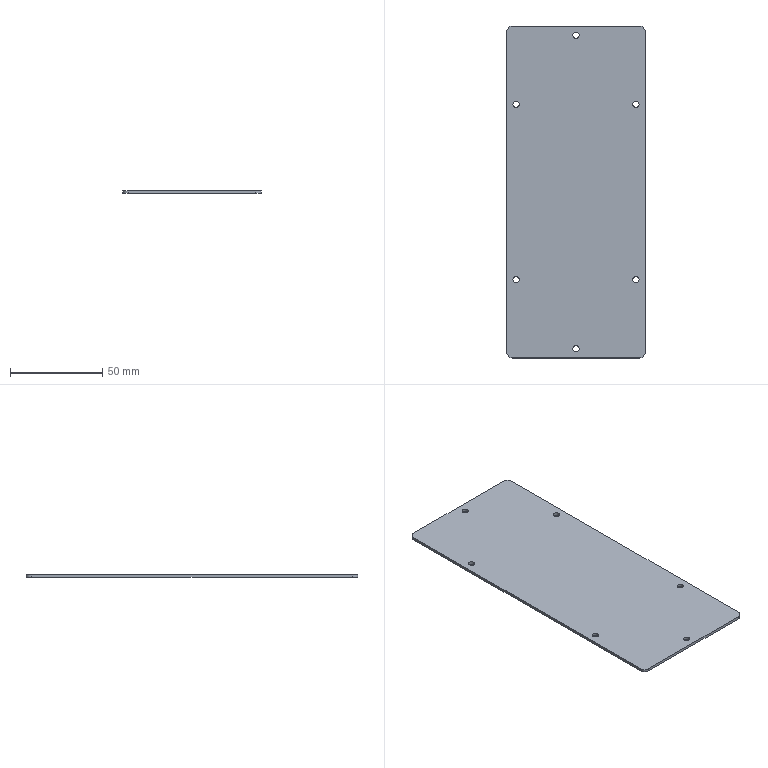Part | NX | 1 solid | 16 faces | box 75 x 180 x 1.5 mm | volume 20157 mm3 | cylinder 10 | plane 6 | commonest cylinder face diameters 3.4 x6 6 x4
STEP:
#1=CARTESIAN_POINT('',(-34.2,47.5,0.));
#2=VERTEX_POINT('',#1);
#3=CARTESIAN_POINT('',(-32.5,47.5,0.));
#4=DIRECTION('',(0.,0.,-1.));
#5=DIRECTION('',(-1.,0.,0.));
#6=AXIS2_PLACEMENT_3D('',#3,#4,#5);
#7=CIRCLE('',#6,1.7);
#8=EDGE_CURVE('',#2,#2,#7,.T.);
#9=ORIENTED_EDGE('',*,*,#8,.F.);
#10=EDGE_LOOP('',(#9));
#11=FACE_BOUND('',#10,.T.);
#12=CARTESIAN_POINT('',(-1.7,-85.,0.));
#13=VERTEX_POINT('',#12);
#14=CARTESIAN_POINT('',(0.,-85.,0.));
#15=DIRECTION('',(0.,0.,-1.));
#16=DIRECTION('',(-1.,0.,0.));
#17=AXIS2_PLACEMENT_3D('',#14,#15,#16);
#18=CIRCLE('',#17,1.7);
#19=EDGE_CURVE('',#13,#13,#18,.T.);
#20=ORIENTED_EDGE('',*,*,#19,.F.);
#21=EDGE_LOOP('',(#20));
#22=FACE_BOUND('',#21,.T.);
#23=CARTESIAN_POINT('',(30.8,47.5,0.));
#24=VERTEX_POINT('',#23);
#25=CARTESIAN_POINT('',(32.5,47.5,0.));
#26=DIRECTION('',(0.,0.,-1.));
#27=DIRECTION('',(-1.,0.,0.));
#28=AXIS2_PLACEMENT_3D('',#25,#26,#27);
#29=CIRCLE('',#28,1.7);
#30=EDGE_CURVE('',#24,#24,#29,.T.);
#31=ORIENTED_EDGE('',*,*,#30,.F.);
#32=EDGE_LOOP('',(#31));
#33=FACE_BOUND('',#32,.T.);
#34=CARTESIAN_POINT('',(37.5,-87.,0.));
#35=VERTEX_POINT('',#34);
#36=CARTESIAN_POINT('',(37.5,87.,0.));
#37=VERTEX_POINT('',#36);
#38=CARTESIAN_POINT('',(37.5,90.,0.));
#39=DIRECTION('',(0.,1.,0.));
#40=VECTOR('',#39,1000.);
#41=LINE('',#38,#40);
#42=EDGE_CURVE('',#35,#37,#41,.T.);
#43=ORIENTED_EDGE('',*,*,#42,.F.);
#44=CARTESIAN_POINT('',(34.5,-90.,0.));
#45=VERTEX_POINT('',#44);
#46=CARTESIAN_POINT('',(34.5,-87.,0.));
#47=DIRECTION('',(0.,0.,1.));
#48=DIRECTION('',(1.,0.,0.));
#49=AXIS2_PLACEMENT_3D('',#46,#47,#48);
#50=CIRCLE('',#49,3.);
#51=EDGE_CURVE('',#35,#45,#50,.F.);
#52=ORIENTED_EDGE('',*,*,#51,.T.);
#53=CARTESIAN_POINT('',(-34.5,-90.,0.));
#54=VERTEX_POINT('',#53);
#55=CARTESIAN_POINT('',(-37.5,-90.,0.));
#56=DIRECTION('',(1.,0.,0.));
#57=VECTOR('',#56,1000.);
#58=LINE('',#55,#57);
#59=EDGE_CURVE('',#54,#45,#58,.T.);
#60=ORIENTED_EDGE('',*,*,#59,.F.);
#61=CARTESIAN_POINT('',(-37.5,-87.,0.));
#62=VERTEX_POINT('',#61);
#63=CARTESIAN_POINT('',(-34.5,-87.,0.));
#64=DIRECTION('',(0.,0.,1.));
#65=DIRECTION('',(1.,0.,0.));
#66=AXIS2_PLACEMENT_3D('',#63,#64,#65);
#67=CIRCLE('',#66,3.);
#68=EDGE_CURVE('',#54,#62,#67,.F.);
#69=ORIENTED_EDGE('',*,*,#68,.T.);
#70=CARTESIAN_POINT('',(-37.5,87.,0.));
#71=VERTEX_POINT('',#70);
#72=CARTESIAN_POINT('',(-37.5,90.,0.));
#73=DIRECTION('',(0.,-1.,0.));
#74=VECTOR('',#73,1000.);
#75=LINE('',#72,#74);
#76=EDGE_CURVE('',#71,#62,#75,.T.);
#77=ORIENTED_EDGE('',*,*,#76,.F.);
#78=CARTESIAN_POINT('',(-34.5,90.,0.));
#79=VERTEX_POINT('',#78);
#80=CARTESIAN_POINT('',(-34.5,87.,0.));
#81=DIRECTION('',(0.,0.,1.));
#82=DIRECTION('',(1.,0.,0.));
#83=AXIS2_PLACEMENT_3D('',#80,#81,#82);
#84=CIRCLE('',#83,3.);
#85=EDGE_CURVE('',#71,#79,#84,.F.);
#86=ORIENTED_EDGE('',*,*,#85,.T.);
#87=CARTESIAN_POINT('',(34.5,90.,0.));
#88=VERTEX_POINT('',#87);
#89=CARTESIAN_POINT('',(-37.5,90.,0.));
#90=DIRECTION('',(-1.,0.,0.));
#91=VECTOR('',#90,1000.);
#92=LINE('',#89,#91);
#93=EDGE_CURVE('',#88,#79,#92,.T.);
#94=ORIENTED_EDGE('',*,*,#93,.F.);
#95=CARTESIAN_POINT('',(34.5,87.,0.));
#96=DIRECTION('',(0.,0.,1.));
#97=DIRECTION('',(1.,0.,0.));
#98=AXIS2_PLACEMENT_3D('',#95,#96,#97);
#99=CIRCLE('',#98,3.);
#100=EDGE_CURVE('',#88,#37,#99,.F.);
#101=ORIENTED_EDGE('',*,*,#100,.T.);
#102=EDGE_LOOP('',(#43,#52,#60,#69,#77,#86,#94,#101));
#103=FACE_BOUND('',#102,.T.);
#104=CARTESIAN_POINT('',(30.8,-47.5,0.));
#105=VERTEX_POINT('',#104);
#106=CARTESIAN_POINT('',(32.5,-47.5,0.));
#107=DIRECTION('',(0.,0.,-1.));
#108=DIRECTION('',(-1.,0.,0.));
#109=AXIS2_PLACEMENT_3D('',#106,#107,#108);
#110=CIRCLE('',#109,1.7);
#111=EDGE_CURVE('',#105,#105,#110,.T.);
#112=ORIENTED_EDGE('',*,*,#111,.F.);
#113=EDGE_LOOP('',(#112));
#114=FACE_BOUND('',#113,.T.);
#115=CARTESIAN_POINT('',(-34.2,-47.5,0.));
#116=VERTEX_POINT('',#115);
#117=CARTESIAN_POINT('',(-32.5,-47.5,0.));
#118=DIRECTION('',(0.,0.,-1.));
#119=DIRECTION('',(-1.,0.,0.));
#120=AXIS2_PLACEMENT_3D('',#117,#118,#119);
#121=CIRCLE('',#120,1.7);
#122=EDGE_CURVE('',#116,#116,#121,.T.);
#123=ORIENTED_EDGE('',*,*,#122,.F.);
#124=EDGE_LOOP('',(#123));
#125=FACE_BOUND('',#124,.T.);
#126=CARTESIAN_POINT('',(-1.7,85.,0.));
#127=VERTEX_POINT('',#126);
#128=CARTESIAN_POINT('',(0.,85.,0.));
#129=DIRECTION('',(0.,0.,-1.));
#130=DIRECTION('',(-1.,0.,0.));
#131=AXIS2_PLACEMENT_3D('',#128,#129,#130);
#132=CIRCLE('',#131,1.7);
#133=EDGE_CURVE('',#127,#127,#132,.T.);
#134=ORIENTED_EDGE('',*,*,#133,.F.);
#135=EDGE_LOOP('',(#134));
#136=FACE_BOUND('',#135,.T.);
#137=CARTESIAN_POINT('',(0.,0.,0.));
#138=DIRECTION('',(0.,0.,1.));
#139=DIRECTION('',(1.,0.,0.));
#140=AXIS2_PLACEMENT_3D('',#137,#138,#139);
#141=PLANE('',#140);
#142=ADVANCED_FACE('',(#11,#22,#33,#103,#114,#125,#136),#141,.F.);
#143=CARTESIAN_POINT('',(37.5,-87.,1.5));
#144=VERTEX_POINT('',#143);
#145=CARTESIAN_POINT('',(37.5,87.,1.5));
#146=VERTEX_POINT('',#145);
#147=CARTESIAN_POINT('',(37.5,90.,1.5));
#148=DIRECTION('',(0.,1.,0.));
#149=VECTOR('',#148,1000.);
#150=LINE('',#147,#149);
#151=EDGE_CURVE('',#144,#146,#150,.T.);
#152=ORIENTED_EDGE('',*,*,#151,.F.);
#153=CARTESIAN_POINT('',(37.5,-87.,1.5));
#154=DIRECTION('',(0.,0.,-1.));
#155=VECTOR('',#154,1000.);
#156=LINE('',#153,#155);
#157=EDGE_CURVE('',#144,#35,#156,.T.);
#158=ORIENTED_EDGE('',*,*,#157,.T.);
#159=ORIENTED_EDGE('',*,*,#42,.T.);
#160=CARTESIAN_POINT('',(37.5,87.,1.5));
#161=DIRECTION('',(0.,0.,-1.));
#162=VECTOR('',#161,1000.);
#163=LINE('',#160,#162);
#164=EDGE_CURVE('',#37,#146,#163,.F.);
#165=ORIENTED_EDGE('',*,*,#164,.T.);
#166=EDGE_LOOP('',(#152,#158,#159,#165));
#167=FACE_BOUND('',#166,.T.);
#168=CARTESIAN_POINT('',(37.5,90.,1.5));
#169=DIRECTION('',(-1.,0.,0.));
#170=DIRECTION('',(0.,-1.,0.));
#171=AXIS2_PLACEMENT_3D('',#168,#169,#170);
#172=PLANE('',#171);
#173=ADVANCED_FACE('',(#167),#172,.F.);
#174=ORIENTED_EDGE('',*,*,#93,.T.);
#175=CARTESIAN_POINT('',(-34.5,90.,1.5));
#176=VERTEX_POINT('',#175);
#177=CARTESIAN_POINT('',(-34.5,90.,1.5));
#178=DIRECTION('',(0.,0.,-1.));
#179=VECTOR('',#178,1000.);
#180=LINE('',#177,#179);
#181=EDGE_CURVE('',#79,#176,#180,.F.);
#182=ORIENTED_EDGE('',*,*,#181,.T.);
#183=CARTESIAN_POINT('',(34.5,90.,1.5));
#184=VERTEX_POINT('',#183);
#185=CARTESIAN_POINT('',(-37.5,90.,1.5));
#186=DIRECTION('',(-1.,0.,0.));
#187=VECTOR('',#186,1000.);
#188=LINE('',#185,#187);
#189=EDGE_CURVE('',#184,#176,#188,.T.);
#190=ORIENTED_EDGE('',*,*,#189,.F.);
#191=CARTESIAN_POINT('',(34.5,90.,1.5));
#192=DIRECTION('',(0.,0.,-1.));
#193=VECTOR('',#192,1000.);
#194=LINE('',#191,#193);
#195=EDGE_CURVE('',#184,#88,#194,.T.);
#196=ORIENTED_EDGE('',*,*,#195,.T.);
#197=EDGE_LOOP('',(#174,#182,#190,#196));
#198=FACE_BOUND('',#197,.T.);
#199=CARTESIAN_POINT('',(-37.5,90.,1.5));
#200=DIRECTION('',(0.,-1.,0.));
#201=DIRECTION('',(0.,0.,-1.));
#202=AXIS2_PLACEMENT_3D('',#199,#200,#201);
#203=PLANE('',#202);
#204=ADVANCED_FACE('',(#198),#203,.F.);
#205=ORIENTED_EDGE('',*,*,#76,.T.);
#206=CARTESIAN_POINT('',(-37.5,-87.,1.5));
#207=VERTEX_POINT('',#206);
#208=CARTESIAN_POINT('',(-37.5,-87.,1.5));
#209=DIRECTION('',(0.,0.,-1.));
#210=VECTOR('',#209,1000.);
#211=LINE('',#208,#210);
#212=EDGE_CURVE('',#62,#207,#211,.F.);
#213=ORIENTED_EDGE('',*,*,#212,.T.);
#214=CARTESIAN_POINT('',(-37.5,87.,1.5));
#215=VERTEX_POINT('',#214);
#216=CARTESIAN_POINT('',(-37.5,90.,1.5));
#217=DIRECTION('',(0.,-1.,0.));
#218=VECTOR('',#217,1000.);
#219=LINE('',#216,#218);
#220=EDGE_CURVE('',#215,#207,#219,.T.);
#221=ORIENTED_EDGE('',*,*,#220,.F.);
#222=CARTESIAN_POINT('',(-37.5,87.,1.5));
#223=DIRECTION('',(0.,0.,-1.));
#224=VECTOR('',#223,1000.);
#225=LINE('',#222,#224);
#226=EDGE_CURVE('',#215,#71,#225,.T.);
#227=ORIENTED_EDGE('',*,*,#226,.T.);
#228=EDGE_LOOP('',(#205,#213,#221,#227));
#229=FACE_BOUND('',#228,.T.);
#230=CARTESIAN_POINT('',(-37.5,90.,1.5));
#231=DIRECTION('',(1.,0.,0.));
#232=DIRECTION('',(0.,1.,0.));
#233=AXIS2_PLACEMENT_3D('',#230,#231,#232);
#234=PLANE('',#233);
#235=ADVANCED_FACE('',(#229),#234,.F.);
#236=ORIENTED_EDGE('',*,*,#59,.T.);
#237=CARTESIAN_POINT('',(34.5,-90.,1.5));
#238=VERTEX_POINT('',#237);
#239=CARTESIAN_POINT('',(34.5,-90.,1.5));
#240=DIRECTION('',(0.,0.,-1.));
#241=VECTOR('',#240,1000.);
#242=LINE('',#239,#241);
#243=EDGE_CURVE('',#45,#238,#242,.F.);
#244=ORIENTED_EDGE('',*,*,#243,.T.);
#245=CARTESIAN_POINT('',(-34.5,-90.,1.5));
#246=VERTEX_POINT('',#245);
#247=CARTESIAN_POINT('',(-37.5,-90.,1.5));
#248=DIRECTION('',(1.,0.,0.));
#249=VECTOR('',#248,1000.);
#250=LINE('',#247,#249);
#251=EDGE_CURVE('',#246,#238,#250,.T.);
#252=ORIENTED_EDGE('',*,*,#251,.F.);
#253=CARTESIAN_POINT('',(-34.5,-90.,1.5));
#254=DIRECTION('',(0.,0.,-1.));
#255=VECTOR('',#254,1000.);
#256=LINE('',#253,#255);
#257=EDGE_CURVE('',#246,#54,#256,.T.);
#258=ORIENTED_EDGE('',*,*,#257,.T.);
#259=EDGE_LOOP('',(#236,#244,#252,#258));
#260=FACE_BOUND('',#259,.T.);
#261=CARTESIAN_POINT('',(-37.5,-90.,1.5));
#262=DIRECTION('',(0.,1.,0.));
#263=DIRECTION('',(0.,0.,1.));
#264=AXIS2_PLACEMENT_3D('',#261,#262,#263);
#265=PLANE('',#264);
#266=ADVANCED_FACE('',(#260),#265,.F.);
#267=CARTESIAN_POINT('',(1.7,85.,1.5));
#268=VERTEX_POINT('',#267);
#269=CARTESIAN_POINT('',(0.,85.,1.5));
#270=DIRECTION('',(0.,0.,1.));
#271=DIRECTION('',(1.,0.,0.));
#272=AXIS2_PLACEMENT_3D('',#269,#270,#271);
#273=CIRCLE('',#272,1.7);
#274=EDGE_CURVE('',#268,#268,#273,.T.);
#275=ORIENTED_EDGE('',*,*,#274,.F.);
#276=EDGE_LOOP('',(#275));
#277=FACE_BOUND('',#276,.T.);
#278=CARTESIAN_POINT('',(-30.8,47.5,1.5));
#279=VERTEX_POINT('',#278);
#280=CARTESIAN_POINT('',(-32.5,47.5,1.5));
#281=DIRECTION('',(0.,0.,1.));
#282=DIRECTION('',(1.,0.,0.));
#283=AXIS2_PLACEMENT_3D('',#280,#281,#282);
#284=CIRCLE('',#283,1.7);
#285=EDGE_CURVE('',#279,#279,#284,.T.);
#286=ORIENTED_EDGE('',*,*,#285,.F.);
#287=EDGE_LOOP('',(#286));
#288=FACE_BOUND('',#287,.T.);
#289=CARTESIAN_POINT('',(-30.8,-47.5,1.5));
#290=VERTEX_POINT('',#289);
#291=CARTESIAN_POINT('',(-32.5,-47.5,1.5));
#292=DIRECTION('',(0.,0.,1.));
#293=DIRECTION('',(1.,0.,0.));
#294=AXIS2_PLACEMENT_3D('',#291,#292,#293);
#295=CIRCLE('',#294,1.7);
#296=EDGE_CURVE('',#290,#290,#295,.T.);
#297=ORIENTED_EDGE('',*,*,#296,.F.);
#298=EDGE_LOOP('',(#297));
#299=FACE_BOUND('',#298,.T.);
#300=CARTESIAN_POINT('',(1.7,-85.,1.5));
#301=VERTEX_POINT('',#300);
#302=CARTESIAN_POINT('',(0.,-85.,1.5));
#303=DIRECTION('',(0.,0.,1.));
#304=DIRECTION('',(1.,0.,0.));
#305=AXIS2_PLACEMENT_3D('',#302,#303,#304);
#306=CIRCLE('',#305,1.7);
#307=EDGE_CURVE('',#301,#301,#306,.T.);
#308=ORIENTED_EDGE('',*,*,#307,.F.);
#309=EDGE_LOOP('',(#308));
#310=FACE_BOUND('',#309,.T.);
#311=CARTESIAN_POINT('',(34.2,-47.5,1.5));
#312=VERTEX_POINT('',#311);
#313=CARTESIAN_POINT('',(32.5,-47.5,1.5));
#314=DIRECTION('',(0.,0.,1.));
#315=DIRECTION('',(1.,0.,0.));
#316=AXIS2_PLACEMENT_3D('',#313,#314,#315);
#317=CIRCLE('',#316,1.7);
#318=EDGE_CURVE('',#312,#312,#317,.T.);
#319=ORIENTED_EDGE('',*,*,#318,.F.);
#320=EDGE_LOOP('',(#319));
#321=FACE_BOUND('',#320,.T.);
#322=CARTESIAN_POINT('',(34.2,47.5,1.5));
#323=VERTEX_POINT('',#322);
#324=CARTESIAN_POINT('',(32.5,47.5,1.5));
#325=DIRECTION('',(0.,0.,1.));
#326=DIRECTION('',(1.,0.,0.));
#327=AXIS2_PLACEMENT_3D('',#324,#325,#326);
#328=CIRCLE('',#327,1.7);
#329=EDGE_CURVE('',#323,#323,#328,.T.);
#330=ORIENTED_EDGE('',*,*,#329,.F.);
#331=EDGE_LOOP('',(#330));
#332=FACE_BOUND('',#331,.T.);
#333=ORIENTED_EDGE('',*,*,#251,.T.);
#334=CARTESIAN_POINT('',(34.5,-87.,1.5));
#335=DIRECTION('',(0.,0.,1.));
#336=DIRECTION('',(1.,0.,0.));
#337=AXIS2_PLACEMENT_3D('',#334,#335,#336);
#338=CIRCLE('',#337,3.);
#339=EDGE_CURVE('',#238,#144,#338,.T.);
#340=ORIENTED_EDGE('',*,*,#339,.T.);
#341=ORIENTED_EDGE('',*,*,#151,.T.);
#342=CARTESIAN_POINT('',(34.5,87.,1.5));
#343=DIRECTION('',(0.,0.,1.));
#344=DIRECTION('',(1.,0.,0.));
#345=AXIS2_PLACEMENT_3D('',#342,#343,#344);
#346=CIRCLE('',#345,3.);
#347=EDGE_CURVE('',#146,#184,#346,.T.);
#348=ORIENTED_EDGE('',*,*,#347,.T.);
#349=ORIENTED_EDGE('',*,*,#189,.T.);
#350=CARTESIAN_POINT('',(-34.5,87.,1.5));
#351=DIRECTION('',(0.,0.,1.));
#352=DIRECTION('',(1.,0.,0.));
#353=AXIS2_PLACEMENT_3D('',#350,#351,#352);
#354=CIRCLE('',#353,3.);
#355=EDGE_CURVE('',#176,#215,#354,.T.);
#356=ORIENTED_EDGE('',*,*,#355,.T.);
#357=ORIENTED_EDGE('',*,*,#220,.T.);
#358=CARTESIAN_POINT('',(-34.5,-87.,1.5));
#359=DIRECTION('',(0.,0.,1.));
#360=DIRECTION('',(1.,0.,0.));
#361=AXIS2_PLACEMENT_3D('',#358,#359,#360);
#362=CIRCLE('',#361,3.);
#363=EDGE_CURVE('',#207,#246,#362,.T.);
#364=ORIENTED_EDGE('',*,*,#363,.T.);
#365=EDGE_LOOP('',(#333,#340,#341,#348,#349,#356,#357,#364));
#366=FACE_BOUND('',#365,.T.);
#367=CARTESIAN_POINT('',(0.,0.,1.5));
#368=DIRECTION('',(0.,0.,1.));
#369=DIRECTION('',(1.,0.,0.));
#370=AXIS2_PLACEMENT_3D('',#367,#368,#369);
#371=PLANE('',#370);
#372=ADVANCED_FACE('',(#277,#288,#299,#310,#321,#332,#366),#371,.T.);
#373=ORIENTED_EDGE('',*,*,#339,.F.);
#374=ORIENTED_EDGE('',*,*,#243,.F.);
#375=ORIENTED_EDGE('',*,*,#51,.F.);
#376=ORIENTED_EDGE('',*,*,#157,.F.);
#377=EDGE_LOOP('',(#373,#374,#375,#376));
#378=FACE_BOUND('',#377,.T.);
#379=CARTESIAN_POINT('',(34.5,-87.,1.5));
#380=DIRECTION('',(0.,0.,-1.));
#381=DIRECTION('',(-1.,0.,0.));
#382=AXIS2_PLACEMENT_3D('',#379,#380,#381);
#383=CYLINDRICAL_SURFACE('',#382,3.);
#384=ADVANCED_FACE('',(#378),#383,.T.);
#385=ORIENTED_EDGE('',*,*,#363,.F.);
#386=ORIENTED_EDGE('',*,*,#212,.F.);
#387=ORIENTED_EDGE('',*,*,#68,.F.);
#388=ORIENTED_EDGE('',*,*,#257,.F.);
#389=EDGE_LOOP('',(#385,#386,#387,#388));
#390=FACE_BOUND('',#389,.T.);
#391=CARTESIAN_POINT('',(-34.5,-87.,1.5));
#392=DIRECTION('',(0.,0.,-1.));
#393=DIRECTION('',(-1.,0.,0.));
#394=AXIS2_PLACEMENT_3D('',#391,#392,#393);
#395=CYLINDRICAL_SURFACE('',#394,3.);
#396=ADVANCED_FACE('',(#390),#395,.T.);
#397=ORIENTED_EDGE('',*,*,#355,.F.);
#398=ORIENTED_EDGE('',*,*,#181,.F.);
#399=ORIENTED_EDGE('',*,*,#85,.F.);
#400=ORIENTED_EDGE('',*,*,#226,.F.);
#401=EDGE_LOOP('',(#397,#398,#399,#400));
#402=FACE_BOUND('',#401,.T.);
#403=CARTESIAN_POINT('',(-34.5,87.,1.5));
#404=DIRECTION('',(0.,0.,-1.));
#405=DIRECTION('',(-1.,0.,0.));
#406=AXIS2_PLACEMENT_3D('',#403,#404,#405);
#407=CYLINDRICAL_SURFACE('',#406,3.);
#408=ADVANCED_FACE('',(#402),#407,.T.);
#409=ORIENTED_EDGE('',*,*,#347,.F.);
#410=ORIENTED_EDGE('',*,*,#164,.F.);
#411=ORIENTED_EDGE('',*,*,#100,.F.);
#412=ORIENTED_EDGE('',*,*,#195,.F.);
#413=EDGE_LOOP('',(#409,#410,#411,#412));
#414=FACE_BOUND('',#413,.T.);
#415=CARTESIAN_POINT('',(34.5,87.,1.5));
#416=DIRECTION('',(0.,0.,-1.));
#417=DIRECTION('',(-1.,0.,0.));
#418=AXIS2_PLACEMENT_3D('',#415,#416,#417);
#419=CYLINDRICAL_SURFACE('',#418,3.);
#420=ADVANCED_FACE('',(#414),#419,.T.);
#421=ORIENTED_EDGE('',*,*,#30,.T.);
#422=EDGE_LOOP('',(#421));
#423=FACE_BOUND('',#422,.T.);
#424=ORIENTED_EDGE('',*,*,#329,.T.);
#425=EDGE_LOOP('',(#424));
#426=FACE_BOUND('',#425,.T.);
#427=CARTESIAN_POINT('',(32.5,47.5,0.));
#428=DIRECTION('',(0.,0.,-1.));
#429=DIRECTION('',(-1.,0.,0.));
#430=AXIS2_PLACEMENT_3D('',#427,#428,#429);
#431=CYLINDRICAL_SURFACE('',#430,1.7);
#432=ADVANCED_FACE('',(#423,#426),#431,.F.);
#433=ORIENTED_EDGE('',*,*,#111,.T.);
#434=EDGE_LOOP('',(#433));
#435=FACE_BOUND('',#434,.T.);
#436=ORIENTED_EDGE('',*,*,#318,.T.);
#437=EDGE_LOOP('',(#436));
#438=FACE_BOUND('',#437,.T.);
#439=CARTESIAN_POINT('',(32.5,-47.5,0.));
#440=DIRECTION('',(0.,0.,-1.));
#441=DIRECTION('',(-1.,0.,0.));
#442=AXIS2_PLACEMENT_3D('',#439,#440,#441);
#443=CYLINDRICAL_SURFACE('',#442,1.7);
#444=ADVANCED_FACE('',(#435,#438),#443,.F.);
#445=ORIENTED_EDGE('',*,*,#19,.T.);
#446=EDGE_LOOP('',(#445));
#447=FACE_BOUND('',#446,.T.);
#448=ORIENTED_EDGE('',*,*,#307,.T.);
#449=EDGE_LOOP('',(#448));
#450=FACE_BOUND('',#449,.T.);
#451=CARTESIAN_POINT('',(0.,-85.,0.));
#452=DIRECTION('',(0.,0.,-1.));
#453=DIRECTION('',(-1.,0.,0.));
#454=AXIS2_PLACEMENT_3D('',#451,#452,#453);
#455=CYLINDRICAL_SURFACE('',#454,1.7);
#456=ADVANCED_FACE('',(#447,#450),#455,.F.);
#457=ORIENTED_EDGE('',*,*,#122,.T.);
#458=EDGE_LOOP('',(#457));
#459=FACE_BOUND('',#458,.T.);
#460=ORIENTED_EDGE('',*,*,#296,.T.);
#461=EDGE_LOOP('',(#460));
#462=FACE_BOUND('',#461,.T.);
#463=CARTESIAN_POINT('',(-32.5,-47.5,0.));
#464=DIRECTION('',(0.,0.,-1.));
#465=DIRECTION('',(-1.,0.,0.));
#466=AXIS2_PLACEMENT_3D('',#463,#464,#465);
#467=CYLINDRICAL_SURFACE('',#466,1.7);
#468=ADVANCED_FACE('',(#459,#462),#467,.F.);
#469=ORIENTED_EDGE('',*,*,#8,.T.);
#470=EDGE_LOOP('',(#469));
#471=FACE_BOUND('',#470,.T.);
#472=ORIENTED_EDGE('',*,*,#285,.T.);
#473=EDGE_LOOP('',(#472));
#474=FACE_BOUND('',#473,.T.);
#475=CARTESIAN_POINT('',(-32.5,47.5,0.));
#476=DIRECTION('',(0.,0.,-1.));
#477=DIRECTION('',(-1.,0.,0.));
#478=AXIS2_PLACEMENT_3D('',#475,#476,#477);
#479=CYLINDRICAL_SURFACE('',#478,1.7);
#480=ADVANCED_FACE('',(#471,#474),#479,.F.);
#481=ORIENTED_EDGE('',*,*,#133,.T.);
#482=EDGE_LOOP('',(#481));
#483=FACE_BOUND('',#482,.T.);
#484=ORIENTED_EDGE('',*,*,#274,.T.);
#485=EDGE_LOOP('',(#484));
#486=FACE_BOUND('',#485,.T.);
#487=CARTESIAN_POINT('',(0.,85.,0.));
#488=DIRECTION('',(0.,0.,-1.));
#489=DIRECTION('',(-1.,0.,0.));
#490=AXIS2_PLACEMENT_3D('',#487,#488,#489);
#491=CYLINDRICAL_SURFACE('',#490,1.7);
#492=ADVANCED_FACE('',(#483,#486),#491,.F.);
#493=CLOSED_SHELL('',(#142,#173,#204,#235,#266,#372,#384,#396,#408,#420,#432,#444,#456,#468,#480,#492));
#494=MANIFOLD_SOLID_BREP('',#493);
#495=(LENGTH_UNIT()NAMED_UNIT(*)SI_UNIT(.MILLI.,.METRE.));
#496=UNCERTAINTY_MEASURE_WITH_UNIT(LENGTH_MEASURE(0.00001),#495,'','');
#497=(NAMED_UNIT(*)PLANE_ANGLE_UNIT()SI_UNIT($,.RADIAN.));
#498=(NAMED_UNIT(*)SI_UNIT($,.STERADIAN.)SOLID_ANGLE_UNIT());
#499=(GEOMETRIC_REPRESENTATION_CONTEXT(3)GLOBAL_UNCERTAINTY_ASSIGNED_CONTEXT((#496))GLOBAL_UNIT_ASSIGNED_CONTEXT((#495,#497,#498))REPRESENTATION_CONTEXT('',''));
#500=ADVANCED_BREP_SHAPE_REPRESENTATION('',(#494),#499);